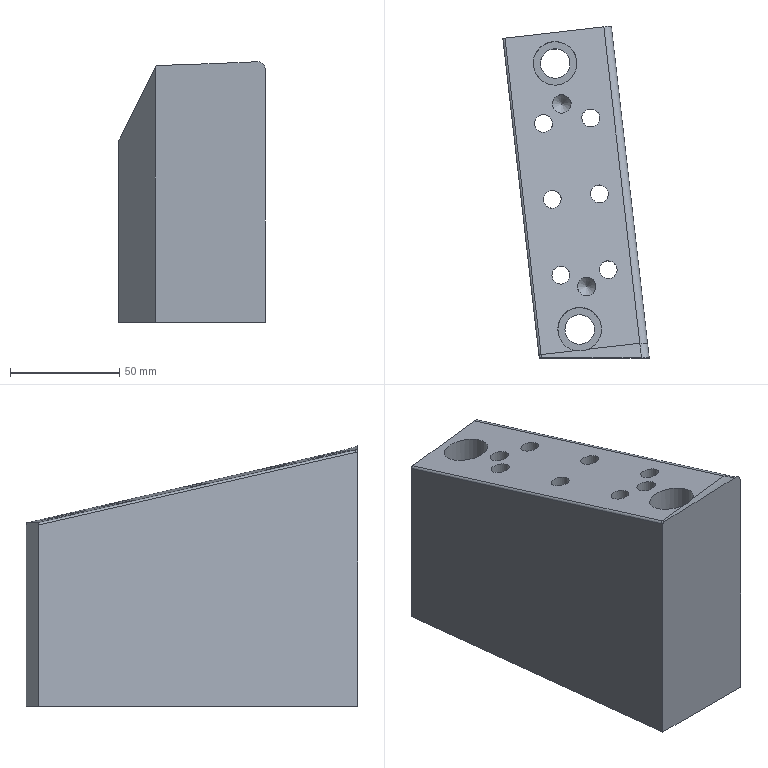Part | NX | features 23 2 | 1 solid | 39 faces | box 66.997 x 151.872 x 119.306 mm | volume 656221 mm3 | cylinder 21 | plane 14 | torus 2 | cone 2 | commonest cylinder face diameters 8.2 x6 10.31 x6 8.5 x2 13.5 x2 20 x2 2 x1
STEP:
#1=CARTESIAN_POINT('',(2421.16,352.401,-62.464));
#2=VERTEX_POINT('',#1);
#3=CARTESIAN_POINT('',(2421.641,348.178,-61.495));
#4=DIRECTION('',(0.02515,-0.2207,-0.975));
#5=DIRECTION('',(-0.1104,0.9687,-0.2221));
#6=AXIS2_PLACEMENT_3D('',#3,#4,#5);
#7=ELLIPSE('',#6,4.359,4.25);
#8=EDGE_CURVE('',#2,#2,#7,.T.);
#9=ORIENTED_EDGE('',*,*,#8,.T.);
#10=EDGE_LOOP('',(#9));
#11=FACE_BOUND('',#10,.T.);
#12=CARTESIAN_POINT('',(2432.577,268.755,-43.235));
#13=VERTEX_POINT('',#12);
#14=CARTESIAN_POINT('',(2433.058,264.532,-42.267));
#15=DIRECTION('',(0.02515,-0.2207,-0.975));
#16=DIRECTION('',(-0.1104,0.9687,-0.2221));
#17=AXIS2_PLACEMENT_3D('',#14,#15,#16);
#18=ELLIPSE('',#17,4.359,4.25);
#19=EDGE_CURVE('',#13,#13,#18,.T.);
#20=ORIENTED_EDGE('',*,*,#19,.T.);
#21=EDGE_LOOP('',(#20));
#22=FACE_BOUND('',#21,.T.);
#23=CARTESIAN_POINT('',(2435.399,337.674,-58.763));
#24=VERTEX_POINT('',#23);
#25=CARTESIAN_POINT('',(2434.935,341.748,-59.697));
#26=DIRECTION('',(-0.02515,0.2207,0.975));
#27=DIRECTION('',(0.1104,-0.9687,0.2221));
#28=AXIS2_PLACEMENT_3D('',#25,#26,#27);
#29=ELLIPSE('',#28,4.205,4.1);
#30=EDGE_CURVE('',#24,#24,#29,.T.);
#31=ORIENTED_EDGE('',*,*,#30,.F.);
#32=EDGE_LOOP('',(#31));
#33=FACE_BOUND('',#32,.T.);
#34=CARTESIAN_POINT('',(2413.764,335.21,-58.763));
#35=VERTEX_POINT('',#34);
#36=CARTESIAN_POINT('',(2413.3,339.283,-59.697));
#37=DIRECTION('',(-0.02515,0.2207,0.975));
#38=DIRECTION('',(0.1104,-0.9687,0.2221));
#39=AXIS2_PLACEMENT_3D('',#36,#37,#38);
#40=ELLIPSE('',#39,4.205,4.1);
#41=EDGE_CURVE('',#35,#35,#40,.T.);
#42=ORIENTED_EDGE('',*,*,#41,.F.);
#43=EDGE_LOOP('',(#42));
#44=FACE_BOUND('',#43,.T.);
#45=CARTESIAN_POINT('',(2439.361,302.899,-50.789));
#46=VERTEX_POINT('',#45);
#47=CARTESIAN_POINT('',(2438.897,306.973,-51.723));
#48=DIRECTION('',(-0.02515,0.2207,0.975));
#49=DIRECTION('',(0.1104,-0.9687,0.2221));
#50=AXIS2_PLACEMENT_3D('',#47,#48,#49);
#51=ELLIPSE('',#50,4.205,4.1);
#52=EDGE_CURVE('',#46,#46,#51,.T.);
#53=ORIENTED_EDGE('',*,*,#52,.F.);
#54=EDGE_LOOP('',(#53));
#55=FACE_BOUND('',#54,.T.);
#56=CARTESIAN_POINT('',(2417.727,300.435,-50.789));
#57=VERTEX_POINT('',#56);
#58=CARTESIAN_POINT('',(2417.262,304.508,-51.723));
#59=DIRECTION('',(-0.02515,0.2207,0.975));
#60=DIRECTION('',(0.1104,-0.9687,0.2221));
#61=AXIS2_PLACEMENT_3D('',#58,#59,#60);
#62=ELLIPSE('',#61,4.205,4.1);
#63=EDGE_CURVE('',#57,#57,#62,.T.);
#64=ORIENTED_EDGE('',*,*,#63,.F.);
#65=EDGE_LOOP('',(#64));
#66=FACE_BOUND('',#65,.T.);
#67=CARTESIAN_POINT('',(2443.323,268.124,-42.815));
#68=VERTEX_POINT('',#67);
#69=CARTESIAN_POINT('',(2442.859,272.198,-43.749));
#70=DIRECTION('',(-0.02515,0.2207,0.975));
#71=DIRECTION('',(0.1104,-0.9687,0.2221));
#72=AXIS2_PLACEMENT_3D('',#69,#70,#71);
#73=ELLIPSE('',#72,4.205,4.1);
#74=EDGE_CURVE('',#68,#68,#73,.T.);
#75=ORIENTED_EDGE('',*,*,#74,.F.);
#76=EDGE_LOOP('',(#75));
#77=FACE_BOUND('',#76,.T.);
#78=CARTESIAN_POINT('',(2421.689,265.66,-42.815));
#79=VERTEX_POINT('',#78);
#80=CARTESIAN_POINT('',(2421.225,269.733,-43.749));
#81=DIRECTION('',(-0.02515,0.2207,0.975));
#82=DIRECTION('',(0.1104,-0.9687,0.2221));
#83=AXIS2_PLACEMENT_3D('',#80,#81,#82);
#84=ELLIPSE('',#83,4.205,4.1);
#85=EDGE_CURVE('',#79,#79,#84,.T.);
#86=ORIENTED_EDGE('',*,*,#85,.F.);
#87=EDGE_LOOP('',(#86));
#88=FACE_BOUND('',#87,.T.);
#89=CARTESIAN_POINT('',(2417.47,376.713,-68.062));
#90=VERTEX_POINT('',#89);
#91=CARTESIAN_POINT('',(2418.602,366.777,-65.784));
#92=DIRECTION('',(-0.02515,0.2207,0.975));
#93=DIRECTION('',(-0.1104,0.9687,-0.2221));
#94=AXIS2_PLACEMENT_3D('',#91,#92,#93);
#95=ELLIPSE('',#94,10.256,10.);
#96=EDGE_CURVE('',#90,#90,#95,.T.);
#97=ORIENTED_EDGE('',*,*,#96,.F.);
#98=EDGE_LOOP('',(#97));
#99=FACE_BOUND('',#98,.T.);
#100=CARTESIAN_POINT('',(2433.88,235.852,-35.754));
#101=VERTEX_POINT('',#100);
#102=CARTESIAN_POINT('',(2457.384,238.53,-35.754));
#103=VERTEX_POINT('',#102);
#104=CARTESIAN_POINT('',(2451.423,237.851,-35.754));
#105=DIRECTION('',(0.9936,0.1132,0.000000001));
#106=VECTOR('',#105,1000.);
#107=LINE('',#104,#106);
#108=EDGE_CURVE('',#101,#103,#107,.T.);
#109=ORIENTED_EDGE('',*,*,#108,.T.);
#110=CARTESIAN_POINT('',(2440.87,383.475,-68.989));
#111=VERTEX_POINT('',#110);
#112=CARTESIAN_POINT('',(2449.818,304.94,-50.981));
#113=DIRECTION('',(-0.1104,0.9687,-0.2221));
#114=VECTOR('',#113,1000.);
#115=LINE('',#112,#114);
#116=EDGE_CURVE('',#103,#111,#115,.T.);
#117=ORIENTED_EDGE('',*,*,#116,.T.);
#118=CARTESIAN_POINT('',(2395.647,378.323,-68.989));
#119=VERTEX_POINT('',#118);
#120=CARTESIAN_POINT('',(2395.583,378.316,-68.989));
#121=DIRECTION('',(0.9936,0.1132,-0.000000001));
#122=VECTOR('',#121,1000.);
#123=LINE('',#120,#122);
#124=EDGE_CURVE('',#119,#111,#123,.T.);
#125=ORIENTED_EDGE('',*,*,#124,.F.);
#126=CARTESIAN_POINT('',(2412.161,233.378,-35.754));
#127=VERTEX_POINT('',#126);
#128=CARTESIAN_POINT('',(2397.033,366.153,-66.199));
#129=DIRECTION('',(-0.1104,0.9687,-0.2221));
#130=VECTOR('',#129,1000.);
#131=LINE('',#128,#130);
#132=EDGE_CURVE('',#127,#119,#131,.T.);
#133=ORIENTED_EDGE('',*,*,#132,.F.);
#134=CARTESIAN_POINT('',(2427.963,235.178,-35.754));
#135=VERTEX_POINT('',#134);
#136=CARTESIAN_POINT('',(2451.423,237.851,-35.754));
#137=DIRECTION('',(0.9936,0.1132,0.000000001));
#138=VECTOR('',#137,1000.);
#139=LINE('',#136,#138);
#140=EDGE_CURVE('',#127,#135,#139,.T.);
#141=ORIENTED_EDGE('',*,*,#140,.T.);
#142=CARTESIAN_POINT('',(2429.841,245.,-37.929));
#143=DIRECTION('',(-0.02515,0.2207,0.975));
#144=DIRECTION('',(-0.1104,0.9687,-0.2221));
#145=AXIS2_PLACEMENT_3D('',#142,#143,#144);
#146=ELLIPSE('',#145,10.256,10.);
#147=EDGE_CURVE('',#101,#135,#146,.T.);
#148=ORIENTED_EDGE('',*,*,#147,.F.);
#149=EDGE_LOOP('',(#109,#117,#125,#133,#141,#148));
#150=FACE_BOUND('',#149,.T.);
#151=CARTESIAN_POINT('',(2449.211,372.098,-66.199));
#152=DIRECTION('',(0.02515,-0.2207,-0.975));
#153=DIRECTION('',(-0.1104,0.9687,-0.2221));
#154=AXIS2_PLACEMENT_3D('',#151,#152,#153);
#155=PLANE('',#154);
#156=ADVANCED_FACE('',(#11,#22,#33,#44,#55,#66,#77,#88,#99,#150),#155,.F.);
#157=CARTESIAN_POINT('',(2394.653,378.21,-70.015));
#158=VERTEX_POINT('',#157);
#159=CARTESIAN_POINT('',(2395.647,378.323,-70.015));
#160=DIRECTION('',(0.1132,-0.9936,0.));
#161=DIRECTION('',(0.,0.,1.));
#162=AXIS2_PLACEMENT_3D('',#159,#160,#161);
#163=ELLIPSE('',#162,1.026,1.);
#164=EDGE_CURVE('',#119,#158,#163,.T.);
#165=ORIENTED_EDGE('',*,*,#164,.F.);
#166=ORIENTED_EDGE('',*,*,#124,.T.);
#167=CARTESIAN_POINT('',(2444.347,383.872,-72.579));
#168=VERTEX_POINT('',#167);
#169=CARTESIAN_POINT('',(2440.87,383.475,-72.579));
#170=DIRECTION('',(0.1132,-0.9936,0.));
#171=DIRECTION('',(0.,0.,1.));
#172=AXIS2_PLACEMENT_3D('',#169,#170,#171);
#173=ELLIPSE('',#172,3.59,3.5);
#174=EDGE_CURVE('',#168,#111,#173,.T.);
#175=ORIENTED_EDGE('',*,*,#174,.F.);
#176=CARTESIAN_POINT('',(2444.347,383.872,-153.));
#177=VERTEX_POINT('',#176);
#178=CARTESIAN_POINT('',(2444.347,383.872,-57.626));
#179=DIRECTION('',(-0.000000001,0.,1.));
#180=VECTOR('',#179,1000.);
#181=LINE('',#178,#180);
#182=EDGE_CURVE('',#177,#168,#181,.T.);
#183=ORIENTED_EDGE('',*,*,#182,.F.);
#184=CARTESIAN_POINT('',(2394.653,378.21,-153.));
#185=VERTEX_POINT('',#184);
#186=CARTESIAN_POINT('',(2395.583,378.316,-153.));
#187=DIRECTION('',(0.9936,0.1132,0.));
#188=VECTOR('',#187,1000.);
#189=LINE('',#186,#188);
#190=EDGE_CURVE('',#185,#177,#189,.T.);
#191=ORIENTED_EDGE('',*,*,#190,.F.);
#192=CARTESIAN_POINT('',(2394.653,378.21,-57.626));
#193=DIRECTION('',(-0.000000002,0.,-1.));
#194=VECTOR('',#193,1000.);
#195=LINE('',#192,#194);
#196=EDGE_CURVE('',#158,#185,#195,.T.);
#197=ORIENTED_EDGE('',*,*,#196,.F.);
#198=EDGE_LOOP('',(#165,#166,#175,#183,#191,#197));
#199=FACE_BOUND('',#198,.T.);
#200=CARTESIAN_POINT('',(2395.583,378.316,-57.626));
#201=DIRECTION('',(-0.1132,0.9936,0.));
#202=DIRECTION('',(0.02514,0.002864,0.9997));
#203=AXIS2_PLACEMENT_3D('',#200,#201,#202);
#204=PLANE('',#203);
#205=ADVANCED_FACE('',(#199),#204,.T.);
#206=CARTESIAN_POINT('',(2411.312,232.,-153.));
#207=VERTEX_POINT('',#206);
#208=CARTESIAN_POINT('',(2411.312,232.,-36.476));
#209=VERTEX_POINT('',#208);
#210=CARTESIAN_POINT('',(2411.312,232.,0.000000275));
#211=DIRECTION('',(0.000000002,0.,1.));
#212=VECTOR('',#211,1000.);
#213=LINE('',#210,#212);
#214=EDGE_CURVE('',#207,#209,#213,.T.);
#215=ORIENTED_EDGE('',*,*,#214,.F.);
#216=CARTESIAN_POINT('',(2461.651,232.,-153.));
#217=VERTEX_POINT('',#216);
#218=CARTESIAN_POINT('',(2566.,232.,-153.));
#219=DIRECTION('',(-1.,0.,0.));
#220=VECTOR('',#219,1000.);
#221=LINE('',#218,#220);
#222=EDGE_CURVE('',#217,#207,#221,.T.);
#223=ORIENTED_EDGE('',*,*,#222,.F.);
#224=CARTESIAN_POINT('',(2461.651,232.,-37.299));
#225=VERTEX_POINT('',#224);
#226=CARTESIAN_POINT('',(2461.651,232.,-0.000000076));
#227=DIRECTION('',(0.000000001,0.,-1.));
#228=VECTOR('',#227,1000.);
#229=LINE('',#226,#228);
#230=EDGE_CURVE('',#225,#217,#229,.T.);
#231=ORIENTED_EDGE('',*,*,#230,.F.);
#232=CARTESIAN_POINT('',(2458.128,232.,-33.697));
#233=VERTEX_POINT('',#232);
#234=CARTESIAN_POINT('',(2458.128,232.,-33.697));
#235=CARTESIAN_POINT('',(2459.076,232.,-33.654));
#236=CARTESIAN_POINT('',(2460.953,232.,-34.457));
#237=CARTESIAN_POINT('',(2461.651,232.,-36.351));
#238=CARTESIAN_POINT('',(2461.651,232.,-37.299));
#239=B_SPLINE_CURVE_WITH_KNOTS('',3,(#234,#235,#236,#237,#238),.UNSPECIFIED.,.F.,.F.,(4,1,4),(0.,0.002806,0.005613),.UNSPECIFIED.);
#240=EDGE_CURVE('',#233,#225,#239,.T.);
#241=ORIENTED_EDGE('',*,*,#240,.F.);
#242=CARTESIAN_POINT('',(2412.318,232.,-35.414));
#243=VERTEX_POINT('',#242);
#244=CARTESIAN_POINT('',(2314.714,232.,6.659));
#245=DIRECTION('',(0.,1.,0.));
#246=DIRECTION('',(1.,0.,0.000000001));
#247=AXIS2_PLACEMENT_3D('',#244,#245,#246);
#248=ELLIPSE('',#247,384.265,43.5);
#249=EDGE_CURVE('',#233,#243,#248,.T.);
#250=ORIENTED_EDGE('',*,*,#249,.T.);
#251=CARTESIAN_POINT('',(2411.312,232.,-36.476));
#252=CARTESIAN_POINT('',(2411.312,232.,-35.932));
#253=CARTESIAN_POINT('',(2411.774,232.,-35.43));
#254=CARTESIAN_POINT('',(2412.318,232.,-35.414));
#255=B_SPLINE_CURVE_WITH_KNOTS('',3,(#251,#252,#253,#254),.UNSPECIFIED.,.F.,.F.,(4,4),(0.,0.001608),.UNSPECIFIED.);
#256=EDGE_CURVE('',#209,#243,#255,.T.);
#257=ORIENTED_EDGE('',*,*,#256,.F.);
#258=EDGE_LOOP('',(#215,#223,#231,#241,#250,#257));
#259=FACE_BOUND('',#258,.T.);
#260=CARTESIAN_POINT('',(2566.,232.,0.));
#261=DIRECTION('',(0.,-1.,0.));
#262=DIRECTION('',(0.,0.,-1.));
#263=AXIS2_PLACEMENT_3D('',#260,#261,#262);
#264=PLANE('',#263);
#265=ADVANCED_FACE('',(#259),#264,.T.);
#266=CARTESIAN_POINT('',(2429.78,341.748,-153.));
#267=VERTEX_POINT('',#266);
#268=CARTESIAN_POINT('',(2434.935,341.748,-153.));
#269=DIRECTION('',(0.,0.,1.));
#270=DIRECTION('',(-1.,0.,0.));
#271=AXIS2_PLACEMENT_3D('',#268,#269,#270);
#272=CIRCLE('',#271,5.155);
#273=EDGE_CURVE('',#267,#267,#272,.T.);
#274=ORIENTED_EDGE('',*,*,#273,.T.);
#275=EDGE_LOOP('',(#274));
#276=FACE_BOUND('',#275,.T.);
#277=CARTESIAN_POINT('',(2408.145,339.283,-153.));
#278=VERTEX_POINT('',#277);
#279=CARTESIAN_POINT('',(2413.3,339.283,-153.));
#280=DIRECTION('',(0.,0.,1.));
#281=DIRECTION('',(-1.,0.,0.));
#282=AXIS2_PLACEMENT_3D('',#279,#280,#281);
#283=CIRCLE('',#282,5.155);
#284=EDGE_CURVE('',#278,#278,#283,.T.);
#285=ORIENTED_EDGE('',*,*,#284,.T.);
#286=EDGE_LOOP('',(#285));
#287=FACE_BOUND('',#286,.T.);
#288=CARTESIAN_POINT('',(2433.742,306.973,-153.));
#289=VERTEX_POINT('',#288);
#290=CARTESIAN_POINT('',(2438.897,306.973,-153.));
#291=DIRECTION('',(0.,0.,1.));
#292=DIRECTION('',(-1.,0.,0.));
#293=AXIS2_PLACEMENT_3D('',#290,#291,#292);
#294=CIRCLE('',#293,5.155);
#295=EDGE_CURVE('',#289,#289,#294,.T.);
#296=ORIENTED_EDGE('',*,*,#295,.T.);
#297=EDGE_LOOP('',(#296));
#298=FACE_BOUND('',#297,.T.);
#299=CARTESIAN_POINT('',(2412.107,304.508,-153.));
#300=VERTEX_POINT('',#299);
#301=CARTESIAN_POINT('',(2417.262,304.508,-153.));
#302=DIRECTION('',(0.,0.,1.));
#303=DIRECTION('',(-1.,0.,0.));
#304=AXIS2_PLACEMENT_3D('',#301,#302,#303);
#305=CIRCLE('',#304,5.155);
#306=EDGE_CURVE('',#300,#300,#305,.T.);
#307=ORIENTED_EDGE('',*,*,#306,.T.);
#308=EDGE_LOOP('',(#307));
#309=FACE_BOUND('',#308,.T.);
#310=CARTESIAN_POINT('',(2437.704,272.198,-153.));
#311=VERTEX_POINT('',#310);
#312=CARTESIAN_POINT('',(2442.859,272.198,-153.));
#313=DIRECTION('',(0.,0.,1.));
#314=DIRECTION('',(-1.,0.,0.));
#315=AXIS2_PLACEMENT_3D('',#312,#313,#314);
#316=CIRCLE('',#315,5.155);
#317=EDGE_CURVE('',#311,#311,#316,.T.);
#318=ORIENTED_EDGE('',*,*,#317,.T.);
#319=EDGE_LOOP('',(#318));
#320=FACE_BOUND('',#319,.T.);
#321=CARTESIAN_POINT('',(2416.07,269.733,-153.));
#322=VERTEX_POINT('',#321);
#323=CARTESIAN_POINT('',(2421.225,269.733,-153.));
#324=DIRECTION('',(0.,0.,1.));
#325=DIRECTION('',(-1.,0.,0.));
#326=AXIS2_PLACEMENT_3D('',#323,#324,#325);
#327=CIRCLE('',#326,5.155);
#328=EDGE_CURVE('',#322,#322,#327,.T.);
#329=ORIENTED_EDGE('',*,*,#328,.T.);
#330=EDGE_LOOP('',(#329));
#331=FACE_BOUND('',#330,.T.);
#332=CARTESIAN_POINT('',(2411.852,366.777,-153.));
#333=VERTEX_POINT('',#332);
#334=CARTESIAN_POINT('',(2418.602,366.777,-153.));
#335=DIRECTION('',(0.,0.,1.));
#336=DIRECTION('',(-1.,0.,0.));
#337=AXIS2_PLACEMENT_3D('',#334,#335,#336);
#338=CIRCLE('',#337,6.75);
#339=EDGE_CURVE('',#333,#333,#338,.T.);
#340=ORIENTED_EDGE('',*,*,#339,.T.);
#341=EDGE_LOOP('',(#340));
#342=FACE_BOUND('',#341,.T.);
#343=CARTESIAN_POINT('',(2423.091,245.,-153.));
#344=VERTEX_POINT('',#343);
#345=CARTESIAN_POINT('',(2429.841,245.,-153.));
#346=DIRECTION('',(0.,0.,1.));
#347=DIRECTION('',(-1.,0.,0.));
#348=AXIS2_PLACEMENT_3D('',#345,#346,#347);
#349=CIRCLE('',#348,6.75);
#350=EDGE_CURVE('',#344,#344,#349,.T.);
#351=ORIENTED_EDGE('',*,*,#350,.T.);
#352=EDGE_LOOP('',(#351));
#353=FACE_BOUND('',#352,.T.);
#354=ORIENTED_EDGE('',*,*,#190,.T.);
#355=CARTESIAN_POINT('',(2481.527,57.547,-153.));
#356=DIRECTION('',(-0.1132,0.9936,0.));
#357=VECTOR('',#356,1000.);
#358=LINE('',#355,#357);
#359=EDGE_CURVE('',#217,#177,#358,.T.);
#360=ORIENTED_EDGE('',*,*,#359,.F.);
#361=ORIENTED_EDGE('',*,*,#222,.T.);
#362=CARTESIAN_POINT('',(2431.833,51.886,-153.));
#363=DIRECTION('',(0.1132,-0.9936,0.));
#364=VECTOR('',#363,1000.);
#365=LINE('',#362,#364);
#366=EDGE_CURVE('',#185,#207,#365,.T.);
#367=ORIENTED_EDGE('',*,*,#366,.F.);
#368=EDGE_LOOP('',(#354,#360,#361,#367));
#369=FACE_BOUND('',#368,.T.);
#370=CARTESIAN_POINT('',(282.5,-193.,-153.));
#371=DIRECTION('',(0.,0.,-1.));
#372=DIRECTION('',(-1.,0.,0.));
#373=AXIS2_PLACEMENT_3D('',#370,#371,#372);
#374=PLANE('',#373);
#375=ADVANCED_FACE('',(#276,#287,#298,#309,#320,#331,#342,#353,#369),#374,.T.);
#376=ORIENTED_EDGE('',*,*,#132,.T.);
#377=ORIENTED_EDGE('',*,*,#164,.T.);
#378=CARTESIAN_POINT('',(2411.193,233.044,-36.729));
#379=VERTEX_POINT('',#378);
#380=CARTESIAN_POINT('',(2396.065,365.819,-67.174));
#381=DIRECTION('',(0.1104,-0.9687,0.2221));
#382=VECTOR('',#381,1000.);
#383=LINE('',#380,#382);
#384=EDGE_CURVE('',#158,#379,#383,.T.);
#385=ORIENTED_EDGE('',*,*,#384,.T.);
#386=CARTESIAN_POINT('',(2412.186,233.157,-36.729));
#387=DIRECTION('',(0.1104,-0.9687,0.2221));
#388=DIRECTION('',(0.,-0.2235,-0.9747));
#389=AXIS2_PLACEMENT_3D('',#386,#387,#388);
#390=CIRCLE('',#389,1.);
#391=EDGE_CURVE('',#127,#379,#390,.T.);
#392=ORIENTED_EDGE('',*,*,#391,.F.);
#393=EDGE_LOOP('',(#376,#377,#385,#392));
#394=FACE_BOUND('',#393,.T.);
#395=CARTESIAN_POINT('',(2397.059,365.932,-67.174));
#396=DIRECTION('',(0.1104,-0.9687,0.2221));
#397=DIRECTION('',(0.,0.2235,0.9747));
#398=AXIS2_PLACEMENT_3D('',#395,#396,#397);
#399=CYLINDRICAL_SURFACE('',#398,1.);
#400=ADVANCED_FACE('',(#394),#399,.T.);
#401=CARTESIAN_POINT('',(2410.074,242.865,6.659));
#402=DIRECTION('',(-0.9936,-0.1132,0.000000002));
#403=DIRECTION('',(-0.1132,0.9936,0.));
#404=AXIS2_PLACEMENT_3D('',#401,#402,#403);
#405=CIRCLE('',#404,44.5);
#406=EDGE_CURVE('',#379,#209,#405,.T.);
#407=ORIENTED_EDGE('',*,*,#406,.F.);
#408=ORIENTED_EDGE('',*,*,#384,.F.);
#409=ORIENTED_EDGE('',*,*,#196,.T.);
#410=ORIENTED_EDGE('',*,*,#366,.T.);
#411=ORIENTED_EDGE('',*,*,#214,.T.);
#412=EDGE_LOOP('',(#407,#408,#409,#410,#411));
#413=FACE_BOUND('',#412,.T.);
#414=CARTESIAN_POINT('',(2411.08,234.037,-32.341));
#415=DIRECTION('',(-0.9936,-0.1132,0.000000002));
#416=DIRECTION('',(0.1132,-0.9936,0.000000002));
#417=AXIS2_PLACEMENT_3D('',#414,#415,#416);
#418=PLANE('',#417);
#419=ADVANCED_FACE('',(#413),#418,.T.);
#420=ORIENTED_EDGE('',*,*,#174,.T.);
#421=ORIENTED_EDGE('',*,*,#116,.F.);
#422=CARTESIAN_POINT('',(2460.95,238.154,-39.166));
#423=VERTEX_POINT('',#422);
#424=CARTESIAN_POINT('',(2457.472,237.758,-39.166));
#425=DIRECTION('',(-0.1104,0.9687,-0.2221));
#426=DIRECTION('',(-0.6687,-0.2377,-0.7045));
#427=AXIS2_PLACEMENT_3D('',#424,#425,#426);
#428=CIRCLE('',#427,3.5);
#429=EDGE_CURVE('',#103,#423,#428,.T.);
#430=ORIENTED_EDGE('',*,*,#429,.T.);
#431=CARTESIAN_POINT('',(2453.383,304.563,-54.394));
#432=DIRECTION('',(0.1104,-0.9687,0.2221));
#433=VECTOR('',#432,1000.);
#434=LINE('',#431,#433);
#435=EDGE_CURVE('',#168,#423,#434,.T.);
#436=ORIENTED_EDGE('',*,*,#435,.F.);
#437=EDGE_LOOP('',(#420,#421,#430,#436));
#438=FACE_BOUND('',#437,.T.);
#439=CARTESIAN_POINT('',(2452.744,279.254,-48.681));
#440=DIRECTION('',(0.1104,-0.9687,0.2221));
#441=DIRECTION('',(0.6848,0.2361,0.6894));
#442=AXIS2_PLACEMENT_3D('',#439,#440,#441);
#443=CYLINDRICAL_SURFACE('',#442,3.5);
#444=ADVANCED_FACE('',(#438),#443,.T.);
#445=ORIENTED_EDGE('',*,*,#435,.T.);
#446=CARTESIAN_POINT('',(2463.469,216.037,-27.1));
#447=CARTESIAN_POINT('',(2462.948,220.611,-31.559));
#448=CARTESIAN_POINT('',(2462.335,225.992,-35.182));
#449=CARTESIAN_POINT('',(2461.657,231.945,-37.743));
#450=CARTESIAN_POINT('',(2460.95,238.154,-39.166));
#451=B_SPLINE_CURVE_WITH_KNOTS('',4,(#446,#447,#448,#449,#450),.UNSPECIFIED.,.F.,.F.,(5,5),(0.,1.),.PIECEWISE_BEZIER_KNOTS.);
#452=EDGE_CURVE('',#225,#423,#451,.T.);
#453=ORIENTED_EDGE('',*,*,#452,.F.);
#454=ORIENTED_EDGE('',*,*,#230,.T.);
#455=ORIENTED_EDGE('',*,*,#359,.T.);
#456=ORIENTED_EDGE('',*,*,#182,.T.);
#457=EDGE_LOOP('',(#445,#453,#454,#455,#456));
#458=FACE_BOUND('',#457,.T.);
#459=CARTESIAN_POINT('',(2310.296,1560.421,-706.6));
#460=DIRECTION('',(0.9936,0.1132,0.000000001));
#461=DIRECTION('',(0.000000001,-0.000000001,-1.));
#462=AXIS2_PLACEMENT_3D('',#459,#460,#461);
#463=PLANE('',#462);
#464=ADVANCED_FACE('',(#458),#463,.T.);
#465=ORIENTED_EDGE('',*,*,#256,.T.);
#466=CARTESIAN_POINT('',(2412.318,232.,-35.414));
#467=CARTESIAN_POINT('',(2412.266,232.457,-35.535));
#468=CARTESIAN_POINT('',(2412.214,232.916,-35.648));
#469=CARTESIAN_POINT('',(2412.161,233.378,-35.754));
#470=B_SPLINE_CURVE_WITH_KNOTS('',3,(#466,#467,#468,#469),.UNSPECIFIED.,.F.,.F.,(4,4),(0.,1.),.PIECEWISE_BEZIER_KNOTS.);
#471=EDGE_CURVE('',#243,#127,#470,.T.);
#472=ORIENTED_EDGE('',*,*,#471,.T.);
#473=ORIENTED_EDGE('',*,*,#391,.T.);
#474=ORIENTED_EDGE('',*,*,#406,.T.);
#475=EDGE_LOOP('',(#465,#472,#473,#474));
#476=FACE_BOUND('',#475,.T.);
#477=CARTESIAN_POINT('',(2411.067,242.978,6.659));
#478=DIRECTION('',(-0.9936,-0.1132,0.000000002));
#479=DIRECTION('',(0.1132,-0.9936,0.));
#480=AXIS2_PLACEMENT_3D('',#477,#478,#479);
#481=TOROIDAL_SURFACE('',#480,44.5,1.);
#482=ADVANCED_FACE('',(#476),#481,.T.);
#483=ORIENTED_EDGE('',*,*,#240,.T.);
#484=ORIENTED_EDGE('',*,*,#452,.T.);
#485=ORIENTED_EDGE('',*,*,#429,.F.);
#486=CARTESIAN_POINT('',(2456.29,248.131,6.659));
#487=DIRECTION('',(-0.9936,-0.1132,-0.000000001));
#488=DIRECTION('',(0.1132,-0.9936,0.000000001));
#489=AXIS2_PLACEMENT_3D('',#486,#487,#488);
#490=CIRCLE('',#489,43.5);
#491=EDGE_CURVE('',#103,#233,#490,.T.);
#492=ORIENTED_EDGE('',*,*,#491,.T.);
#493=EDGE_LOOP('',(#483,#484,#485,#492));
#494=FACE_BOUND('',#493,.T.);
#495=CARTESIAN_POINT('',(2456.29,248.131,6.659));
#496=DIRECTION('',(0.9936,0.1132,0.000000001));
#497=DIRECTION('',(0.05395,-0.4735,-0.8791));
#498=AXIS2_PLACEMENT_3D('',#495,#496,#497);
#499=TOROIDAL_SURFACE('',#498,47.,3.5);
#500=ADVANCED_FACE('',(#494),#499,.T.);
#501=ORIENTED_EDGE('',*,*,#140,.F.);
#502=ORIENTED_EDGE('',*,*,#471,.F.);
#503=ORIENTED_EDGE('',*,*,#249,.F.);
#504=ORIENTED_EDGE('',*,*,#491,.F.);
#505=ORIENTED_EDGE('',*,*,#108,.F.);
#506=CARTESIAN_POINT('',(2427.963,235.178,-35.754));
#507=CARTESIAN_POINT('',(2429.956,234.797,-35.616));
#508=CARTESIAN_POINT('',(2432.024,235.032,-35.616));
#509=CARTESIAN_POINT('',(2433.88,235.852,-35.754));
#510=B_SPLINE_CURVE_WITH_KNOTS('',3,(#506,#507,#508,#509),.UNSPECIFIED.,.F.,.F.,(4,4),(0.,0.006016),.UNSPECIFIED.);
#511=EDGE_CURVE('',#135,#101,#510,.T.);
#512=ORIENTED_EDGE('',*,*,#511,.F.);
#513=EDGE_LOOP('',(#501,#502,#503,#504,#505,#512));
#514=FACE_BOUND('',#513,.T.);
#515=CARTESIAN_POINT('',(2445.361,246.885,6.659));
#516=DIRECTION('',(0.9936,0.1132,0.000000001));
#517=DIRECTION('',(0.08782,-0.7708,-0.631));
#518=AXIS2_PLACEMENT_3D('',#515,#516,#517);
#519=CYLINDRICAL_SURFACE('',#518,43.5);
#520=ADVANCED_FACE('',(#514),#519,.F.);
#521=CARTESIAN_POINT('',(2439.841,245.,-123.));
#522=VERTEX_POINT('',#521);
#523=CARTESIAN_POINT('',(2429.841,245.,-123.));
#524=DIRECTION('',(0.,0.,1.));
#525=DIRECTION('',(1.,0.,0.));
#526=AXIS2_PLACEMENT_3D('',#523,#524,#525);
#527=CIRCLE('',#526,10.);
#528=EDGE_CURVE('',#522,#522,#527,.T.);
#529=ORIENTED_EDGE('',*,*,#528,.F.);
#530=EDGE_LOOP('',(#529));
#531=FACE_BOUND('',#530,.T.);
#532=ORIENTED_EDGE('',*,*,#511,.T.);
#533=ORIENTED_EDGE('',*,*,#147,.T.);
#534=EDGE_LOOP('',(#532,#533));
#535=FACE_BOUND('',#534,.T.);
#536=CARTESIAN_POINT('',(2429.841,245.,-33.507));
#537=DIRECTION('',(0.,0.,-1.));
#538=DIRECTION('',(-1.,0.,0.));
#539=AXIS2_PLACEMENT_3D('',#536,#537,#538);
#540=CYLINDRICAL_SURFACE('',#539,10.);
#541=ADVANCED_FACE('',(#531,#535),#540,.F.);
#542=ORIENTED_EDGE('',*,*,#350,.F.);
#543=EDGE_LOOP('',(#542));
#544=FACE_BOUND('',#543,.T.);
#545=CARTESIAN_POINT('',(2436.591,245.,-123.));
#546=VERTEX_POINT('',#545);
#547=CARTESIAN_POINT('',(2429.841,245.,-123.));
#548=DIRECTION('',(0.,0.,1.));
#549=DIRECTION('',(1.,0.,0.));
#550=AXIS2_PLACEMENT_3D('',#547,#548,#549);
#551=CIRCLE('',#550,6.75);
#552=EDGE_CURVE('',#546,#546,#551,.T.);
#553=ORIENTED_EDGE('',*,*,#552,.T.);
#554=EDGE_LOOP('',(#553));
#555=FACE_BOUND('',#554,.T.);
#556=CARTESIAN_POINT('',(2429.841,245.,-28.507));
#557=DIRECTION('',(0.,0.,-1.));
#558=DIRECTION('',(-1.,0.,0.));
#559=AXIS2_PLACEMENT_3D('',#556,#557,#558);
#560=CYLINDRICAL_SURFACE('',#559,6.75);
#561=ADVANCED_FACE('',(#544,#555),#560,.F.);
#562=ORIENTED_EDGE('',*,*,#552,.F.);
#563=EDGE_LOOP('',(#562));
#564=FACE_BOUND('',#563,.T.);
#565=ORIENTED_EDGE('',*,*,#528,.T.);
#566=EDGE_LOOP('',(#565));
#567=FACE_BOUND('',#566,.T.);
#568=CARTESIAN_POINT('',(2429.841,245.,-123.));
#569=DIRECTION('',(0.,0.,-1.));
#570=DIRECTION('',(-1.,0.,0.));
#571=AXIS2_PLACEMENT_3D('',#568,#569,#570);
#572=PLANE('',#571);
#573=ADVANCED_FACE('',(#564,#567),#572,.F.);
#574=CARTESIAN_POINT('',(2428.602,366.777,-123.));
#575=VERTEX_POINT('',#574);
#576=CARTESIAN_POINT('',(2418.602,366.777,-123.));
#577=DIRECTION('',(0.,0.,1.));
#578=DIRECTION('',(1.,0.,0.));
#579=AXIS2_PLACEMENT_3D('',#576,#577,#578);
#580=CIRCLE('',#579,10.);
#581=EDGE_CURVE('',#575,#575,#580,.T.);
#582=ORIENTED_EDGE('',*,*,#581,.F.);
#583=EDGE_LOOP('',(#582));
#584=FACE_BOUND('',#583,.T.);
#585=ORIENTED_EDGE('',*,*,#96,.T.);
#586=EDGE_LOOP('',(#585));
#587=FACE_BOUND('',#586,.T.);
#588=CARTESIAN_POINT('',(2418.602,366.777,-33.507));
#589=DIRECTION('',(0.,0.,-1.));
#590=DIRECTION('',(-1.,0.,0.));
#591=AXIS2_PLACEMENT_3D('',#588,#589,#590);
#592=CYLINDRICAL_SURFACE('',#591,10.);
#593=ADVANCED_FACE('',(#584,#587),#592,.F.);
#594=ORIENTED_EDGE('',*,*,#339,.F.);
#595=EDGE_LOOP('',(#594));
#596=FACE_BOUND('',#595,.T.);
#597=CARTESIAN_POINT('',(2425.352,366.777,-123.));
#598=VERTEX_POINT('',#597);
#599=CARTESIAN_POINT('',(2418.602,366.777,-123.));
#600=DIRECTION('',(0.,0.,1.));
#601=DIRECTION('',(1.,0.,0.));
#602=AXIS2_PLACEMENT_3D('',#599,#600,#601);
#603=CIRCLE('',#602,6.75);
#604=EDGE_CURVE('',#598,#598,#603,.T.);
#605=ORIENTED_EDGE('',*,*,#604,.T.);
#606=EDGE_LOOP('',(#605));
#607=FACE_BOUND('',#606,.T.);
#608=CARTESIAN_POINT('',(2418.602,366.777,-28.507));
#609=DIRECTION('',(0.,0.,-1.));
#610=DIRECTION('',(-1.,0.,0.));
#611=AXIS2_PLACEMENT_3D('',#608,#609,#610);
#612=CYLINDRICAL_SURFACE('',#611,6.75);
#613=ADVANCED_FACE('',(#596,#607),#612,.F.);
#614=ORIENTED_EDGE('',*,*,#604,.F.);
#615=EDGE_LOOP('',(#614));
#616=FACE_BOUND('',#615,.T.);
#617=ORIENTED_EDGE('',*,*,#581,.T.);
#618=EDGE_LOOP('',(#617));
#619=FACE_BOUND('',#618,.T.);
#620=CARTESIAN_POINT('',(2418.602,366.777,-123.));
#621=DIRECTION('',(0.,0.,-1.));
#622=DIRECTION('',(-1.,0.,0.));
#623=AXIS2_PLACEMENT_3D('',#620,#621,#622);
#624=PLANE('',#623);
#625=ADVANCED_FACE('',(#616,#619),#624,.F.);
#626=CARTESIAN_POINT('',(2417.125,269.733,-72.8));
#627=VERTEX_POINT('',#626);
#628=CARTESIAN_POINT('',(2421.225,269.733,-72.8));
#629=DIRECTION('',(0.000000001,0.,-1.));
#630=DIRECTION('',(-1.,0.000000001,-0.000000001));
#631=AXIS2_PLACEMENT_3D('',#628,#629,#630);
#632=CIRCLE('',#631,4.1);
#633=EDGE_CURVE('',#627,#627,#632,.T.);
#634=ORIENTED_EDGE('',*,*,#633,.T.);
#635=EDGE_LOOP('',(#634));
#636=FACE_BOUND('',#635,.T.);
#637=ORIENTED_EDGE('',*,*,#85,.T.);
#638=EDGE_LOOP('',(#637));
#639=FACE_BOUND('',#638,.T.);
#640=CARTESIAN_POINT('',(2421.225,269.733,-75.8));
#641=DIRECTION('',(-0.000000001,0.,1.));
#642=DIRECTION('',(1.,-0.000000001,0.000000001));
#643=AXIS2_PLACEMENT_3D('',#640,#641,#642);
#644=CYLINDRICAL_SURFACE('',#643,4.1);
#645=ADVANCED_FACE('',(#636,#639),#644,.F.);
#646=ORIENTED_EDGE('',*,*,#633,.F.);
#647=EDGE_LOOP('',(#646));
#648=FACE_BOUND('',#647,.T.);
#649=CARTESIAN_POINT('',(2426.38,269.733,-72.8));
#650=VERTEX_POINT('',#649);
#651=CARTESIAN_POINT('',(2421.225,269.733,-72.8));
#652=DIRECTION('',(0.000000001,0.,-1.));
#653=DIRECTION('',(1.,0.,0.000000001));
#654=AXIS2_PLACEMENT_3D('',#651,#652,#653);
#655=CIRCLE('',#654,5.155);
#656=EDGE_CURVE('',#650,#650,#655,.T.);
#657=ORIENTED_EDGE('',*,*,#656,.T.);
#658=EDGE_LOOP('',(#657));
#659=FACE_BOUND('',#658,.T.);
#660=CARTESIAN_POINT('',(2421.225,269.733,-72.8));
#661=DIRECTION('',(-0.000000001,0.,1.));
#662=DIRECTION('',(1.,-0.000000001,0.000000001));
#663=AXIS2_PLACEMENT_3D('',#660,#661,#662);
#664=PLANE('',#663);
#665=ADVANCED_FACE('',(#648,#659),#664,.F.);
#666=ORIENTED_EDGE('',*,*,#328,.F.);
#667=EDGE_LOOP('',(#666));
#668=FACE_BOUND('',#667,.T.);
#669=ORIENTED_EDGE('',*,*,#656,.F.);
#670=EDGE_LOOP('',(#669));
#671=FACE_BOUND('',#670,.T.);
#672=CARTESIAN_POINT('',(2421.225,269.733,-72.8));
#673=DIRECTION('',(0.000000001,0.,-1.));
#674=DIRECTION('',(1.,-0.000000001,0.000000001));
#675=AXIS2_PLACEMENT_3D('',#672,#673,#674);
#676=CYLINDRICAL_SURFACE('',#675,5.155);
#677=ADVANCED_FACE('',(#668,#671),#676,.F.);
#678=CARTESIAN_POINT('',(2446.854,273.12,-72.8));
#679=VERTEX_POINT('',#678);
#680=CARTESIAN_POINT('',(2442.859,272.198,-72.8));
#681=DIRECTION('',(0.,0.,1.));
#682=DIRECTION('',(0.9744,0.225,0.));
#683=AXIS2_PLACEMENT_3D('',#680,#681,#682);
#684=CIRCLE('',#683,4.1);
#685=EDGE_CURVE('',#679,#679,#684,.T.);
#686=ORIENTED_EDGE('',*,*,#685,.F.);
#687=EDGE_LOOP('',(#686));
#688=FACE_BOUND('',#687,.T.);
#689=ORIENTED_EDGE('',*,*,#74,.T.);
#690=EDGE_LOOP('',(#689));
#691=FACE_BOUND('',#690,.T.);
#692=CARTESIAN_POINT('',(2442.859,272.198,-75.8));
#693=DIRECTION('',(0.,0.,1.));
#694=DIRECTION('',(-0.9744,-0.225,0.));
#695=AXIS2_PLACEMENT_3D('',#692,#693,#694);
#696=CYLINDRICAL_SURFACE('',#695,4.1);
#697=ADVANCED_FACE('',(#688,#691),#696,.F.);
#698=ORIENTED_EDGE('',*,*,#685,.T.);
#699=EDGE_LOOP('',(#698));
#700=FACE_BOUND('',#699,.T.);
#701=CARTESIAN_POINT('',(2448.014,272.198,-72.8));
#702=VERTEX_POINT('',#701);
#703=CARTESIAN_POINT('',(2442.859,272.198,-72.8));
#704=DIRECTION('',(0.,0.,1.));
#705=DIRECTION('',(1.,0.,0.));
#706=AXIS2_PLACEMENT_3D('',#703,#704,#705);
#707=CIRCLE('',#706,5.155);
#708=EDGE_CURVE('',#702,#702,#707,.T.);
#709=ORIENTED_EDGE('',*,*,#708,.F.);
#710=EDGE_LOOP('',(#709));
#711=FACE_BOUND('',#710,.T.);
#712=CARTESIAN_POINT('',(2442.859,272.198,-72.8));
#713=DIRECTION('',(0.,0.,1.));
#714=DIRECTION('',(-0.9744,-0.225,0.));
#715=AXIS2_PLACEMENT_3D('',#712,#713,#714);
#716=PLANE('',#715);
#717=ADVANCED_FACE('',(#700,#711),#716,.F.);
#718=ORIENTED_EDGE('',*,*,#317,.F.);
#719=EDGE_LOOP('',(#718));
#720=FACE_BOUND('',#719,.T.);
#721=ORIENTED_EDGE('',*,*,#708,.T.);
#722=EDGE_LOOP('',(#721));
#723=FACE_BOUND('',#722,.T.);
#724=CARTESIAN_POINT('',(2442.859,272.198,-72.8));
#725=DIRECTION('',(0.,0.,-1.));
#726=DIRECTION('',(-0.9744,-0.225,0.));
#727=AXIS2_PLACEMENT_3D('',#724,#725,#726);
#728=CYLINDRICAL_SURFACE('',#727,5.155);
#729=ADVANCED_FACE('',(#720,#723),#728,.F.);
#730=CARTESIAN_POINT('',(2413.267,303.586,-80.8));
#731=VERTEX_POINT('',#730);
#732=CARTESIAN_POINT('',(2417.262,304.508,-80.8));
#733=DIRECTION('',(-0.000000001,0.,1.));
#734=DIRECTION('',(-0.9744,-0.225,-0.000000001));
#735=AXIS2_PLACEMENT_3D('',#732,#733,#734);
#736=CIRCLE('',#735,4.1);
#737=EDGE_CURVE('',#731,#731,#736,.T.);
#738=ORIENTED_EDGE('',*,*,#737,.F.);
#739=EDGE_LOOP('',(#738));
#740=FACE_BOUND('',#739,.T.);
#741=ORIENTED_EDGE('',*,*,#63,.T.);
#742=EDGE_LOOP('',(#741));
#743=FACE_BOUND('',#742,.T.);
#744=CARTESIAN_POINT('',(2417.262,304.508,-83.8));
#745=DIRECTION('',(-0.000000001,0.,1.));
#746=DIRECTION('',(0.9744,0.225,0.000000001));
#747=AXIS2_PLACEMENT_3D('',#744,#745,#746);
#748=CYLINDRICAL_SURFACE('',#747,4.1);
#749=ADVANCED_FACE('',(#740,#743),#748,.F.);
#750=ORIENTED_EDGE('',*,*,#737,.T.);
#751=EDGE_LOOP('',(#750));
#752=FACE_BOUND('',#751,.T.);
#753=CARTESIAN_POINT('',(2422.417,304.508,-80.8));
#754=VERTEX_POINT('',#753);
#755=CARTESIAN_POINT('',(2417.262,304.508,-80.8));
#756=DIRECTION('',(-0.000000001,0.,1.));
#757=DIRECTION('',(1.,0.,0.000000001));
#758=AXIS2_PLACEMENT_3D('',#755,#756,#757);
#759=CIRCLE('',#758,5.155);
#760=EDGE_CURVE('',#754,#754,#759,.T.);
#761=ORIENTED_EDGE('',*,*,#760,.F.);
#762=EDGE_LOOP('',(#761));
#763=FACE_BOUND('',#762,.T.);
#764=CARTESIAN_POINT('',(2417.262,304.508,-80.8));
#765=DIRECTION('',(-0.000000001,0.,1.));
#766=DIRECTION('',(0.9744,0.225,0.000000001));
#767=AXIS2_PLACEMENT_3D('',#764,#765,#766);
#768=PLANE('',#767);
#769=ADVANCED_FACE('',(#752,#763),#768,.F.);
#770=ORIENTED_EDGE('',*,*,#306,.F.);
#771=EDGE_LOOP('',(#770));
#772=FACE_BOUND('',#771,.T.);
#773=ORIENTED_EDGE('',*,*,#760,.T.);
#774=EDGE_LOOP('',(#773));
#775=FACE_BOUND('',#774,.T.);
#776=CARTESIAN_POINT('',(2417.262,304.508,-80.8));
#777=DIRECTION('',(0.000000001,0.,-1.));
#778=DIRECTION('',(0.9744,0.225,0.000000001));
#779=AXIS2_PLACEMENT_3D('',#776,#777,#778);
#780=CYLINDRICAL_SURFACE('',#779,5.155);
#781=ADVANCED_FACE('',(#772,#775),#780,.F.);
#782=CARTESIAN_POINT('',(2442.997,306.973,-80.8));
#783=VERTEX_POINT('',#782);
#784=CARTESIAN_POINT('',(2438.897,306.973,-80.8));
#785=DIRECTION('',(0.,0.,-1.));
#786=DIRECTION('',(1.,0.,0.));
#787=AXIS2_PLACEMENT_3D('',#784,#785,#786);
#788=CIRCLE('',#787,4.1);
#789=EDGE_CURVE('',#783,#783,#788,.T.);
#790=ORIENTED_EDGE('',*,*,#789,.T.);
#791=EDGE_LOOP('',(#790));
#792=FACE_BOUND('',#791,.T.);
#793=ORIENTED_EDGE('',*,*,#52,.T.);
#794=EDGE_LOOP('',(#793));
#795=FACE_BOUND('',#794,.T.);
#796=CARTESIAN_POINT('',(2438.897,306.973,-83.8));
#797=DIRECTION('',(0.,0.,1.));
#798=DIRECTION('',(-1.,0.,0.));
#799=AXIS2_PLACEMENT_3D('',#796,#797,#798);
#800=CYLINDRICAL_SURFACE('',#799,4.1);
#801=ADVANCED_FACE('',(#792,#795),#800,.F.);
#802=ORIENTED_EDGE('',*,*,#789,.F.);
#803=EDGE_LOOP('',(#802));
#804=FACE_BOUND('',#803,.T.);
#805=CARTESIAN_POINT('',(2444.052,306.973,-80.8));
#806=VERTEX_POINT('',#805);
#807=CARTESIAN_POINT('',(2438.897,306.973,-80.8));
#808=DIRECTION('',(0.,0.,-1.));
#809=DIRECTION('',(1.,0.,0.));
#810=AXIS2_PLACEMENT_3D('',#807,#808,#809);
#811=CIRCLE('',#810,5.155);
#812=EDGE_CURVE('',#806,#806,#811,.T.);
#813=ORIENTED_EDGE('',*,*,#812,.T.);
#814=EDGE_LOOP('',(#813));
#815=FACE_BOUND('',#814,.T.);
#816=CARTESIAN_POINT('',(2438.897,306.973,-80.8));
#817=DIRECTION('',(0.,0.,1.));
#818=DIRECTION('',(-1.,0.,0.));
#819=AXIS2_PLACEMENT_3D('',#816,#817,#818);
#820=PLANE('',#819);
#821=ADVANCED_FACE('',(#804,#815),#820,.F.);
#822=ORIENTED_EDGE('',*,*,#295,.F.);
#823=EDGE_LOOP('',(#822));
#824=FACE_BOUND('',#823,.T.);
#825=ORIENTED_EDGE('',*,*,#812,.F.);
#826=EDGE_LOOP('',(#825));
#827=FACE_BOUND('',#826,.T.);
#828=CARTESIAN_POINT('',(2438.897,306.973,-80.8));
#829=DIRECTION('',(0.,0.,-1.));
#830=DIRECTION('',(-1.,0.,0.));
#831=AXIS2_PLACEMENT_3D('',#828,#829,#830);
#832=CYLINDRICAL_SURFACE('',#831,5.155);
#833=ADVANCED_FACE('',(#824,#827),#832,.F.);
#834=CARTESIAN_POINT('',(2409.305,338.361,-88.8));
#835=VERTEX_POINT('',#834);
#836=CARTESIAN_POINT('',(2413.3,339.283,-88.8));
#837=DIRECTION('',(-0.000000001,0.,1.));
#838=DIRECTION('',(-0.9744,-0.225,-0.000000001));
#839=AXIS2_PLACEMENT_3D('',#836,#837,#838);
#840=CIRCLE('',#839,4.1);
#841=EDGE_CURVE('',#835,#835,#840,.T.);
#842=ORIENTED_EDGE('',*,*,#841,.F.);
#843=EDGE_LOOP('',(#842));
#844=FACE_BOUND('',#843,.T.);
#845=ORIENTED_EDGE('',*,*,#41,.T.);
#846=EDGE_LOOP('',(#845));
#847=FACE_BOUND('',#846,.T.);
#848=CARTESIAN_POINT('',(2413.3,339.283,-91.8));
#849=DIRECTION('',(-0.000000001,0.,1.));
#850=DIRECTION('',(0.9744,0.225,0.000000001));
#851=AXIS2_PLACEMENT_3D('',#848,#849,#850);
#852=CYLINDRICAL_SURFACE('',#851,4.1);
#853=ADVANCED_FACE('',(#844,#847),#852,.F.);
#854=ORIENTED_EDGE('',*,*,#841,.T.);
#855=EDGE_LOOP('',(#854));
#856=FACE_BOUND('',#855,.T.);
#857=CARTESIAN_POINT('',(2418.455,339.283,-88.8));
#858=VERTEX_POINT('',#857);
#859=CARTESIAN_POINT('',(2413.3,339.283,-88.8));
#860=DIRECTION('',(-0.000000001,0.,1.));
#861=DIRECTION('',(1.,0.,0.000000001));
#862=AXIS2_PLACEMENT_3D('',#859,#860,#861);
#863=CIRCLE('',#862,5.155);
#864=EDGE_CURVE('',#858,#858,#863,.T.);
#865=ORIENTED_EDGE('',*,*,#864,.F.);
#866=EDGE_LOOP('',(#865));
#867=FACE_BOUND('',#866,.T.);
#868=CARTESIAN_POINT('',(2413.3,339.283,-88.8));
#869=DIRECTION('',(-0.000000001,0.,1.));
#870=DIRECTION('',(0.9744,0.225,0.000000001));
#871=AXIS2_PLACEMENT_3D('',#868,#869,#870);
#872=PLANE('',#871);
#873=ADVANCED_FACE('',(#856,#867),#872,.F.);
#874=ORIENTED_EDGE('',*,*,#284,.F.);
#875=EDGE_LOOP('',(#874));
#876=FACE_BOUND('',#875,.T.);
#877=ORIENTED_EDGE('',*,*,#864,.T.);
#878=EDGE_LOOP('',(#877));
#879=FACE_BOUND('',#878,.T.);
#880=CARTESIAN_POINT('',(2413.3,339.283,-88.8));
#881=DIRECTION('',(0.000000001,0.,-1.));
#882=DIRECTION('',(0.9744,0.225,0.000000001));
#883=AXIS2_PLACEMENT_3D('',#880,#881,#882);
#884=CYLINDRICAL_SURFACE('',#883,5.155);
#885=ADVANCED_FACE('',(#876,#879),#884,.F.);
#886=CARTESIAN_POINT('',(2439.035,341.748,-88.8));
#887=VERTEX_POINT('',#886);
#888=CARTESIAN_POINT('',(2434.935,341.748,-88.8));
#889=DIRECTION('',(0.,0.,-1.));
#890=DIRECTION('',(1.,0.,0.));
#891=AXIS2_PLACEMENT_3D('',#888,#889,#890);
#892=CIRCLE('',#891,4.1);
#893=EDGE_CURVE('',#887,#887,#892,.T.);
#894=ORIENTED_EDGE('',*,*,#893,.T.);
#895=EDGE_LOOP('',(#894));
#896=FACE_BOUND('',#895,.T.);
#897=ORIENTED_EDGE('',*,*,#30,.T.);
#898=EDGE_LOOP('',(#897));
#899=FACE_BOUND('',#898,.T.);
#900=CARTESIAN_POINT('',(2434.935,341.748,-91.8));
#901=DIRECTION('',(0.,0.,1.));
#902=DIRECTION('',(-1.,0.,0.));
#903=AXIS2_PLACEMENT_3D('',#900,#901,#902);
#904=CYLINDRICAL_SURFACE('',#903,4.1);
#905=ADVANCED_FACE('',(#896,#899),#904,.F.);
#906=ORIENTED_EDGE('',*,*,#893,.F.);
#907=EDGE_LOOP('',(#906));
#908=FACE_BOUND('',#907,.T.);
#909=CARTESIAN_POINT('',(2440.09,341.748,-88.8));
#910=VERTEX_POINT('',#909);
#911=CARTESIAN_POINT('',(2434.935,341.748,-88.8));
#912=DIRECTION('',(0.,0.,-1.));
#913=DIRECTION('',(1.,0.,0.));
#914=AXIS2_PLACEMENT_3D('',#911,#912,#913);
#915=CIRCLE('',#914,5.155);
#916=EDGE_CURVE('',#910,#910,#915,.T.);
#917=ORIENTED_EDGE('',*,*,#916,.T.);
#918=EDGE_LOOP('',(#917));
#919=FACE_BOUND('',#918,.T.);
#920=CARTESIAN_POINT('',(2434.935,341.748,-88.8));
#921=DIRECTION('',(0.,0.,1.));
#922=DIRECTION('',(-1.,0.,0.));
#923=AXIS2_PLACEMENT_3D('',#920,#921,#922);
#924=PLANE('',#923);
#925=ADVANCED_FACE('',(#908,#919),#924,.F.);
#926=ORIENTED_EDGE('',*,*,#273,.F.);
#927=EDGE_LOOP('',(#926));
#928=FACE_BOUND('',#927,.T.);
#929=ORIENTED_EDGE('',*,*,#916,.F.);
#930=EDGE_LOOP('',(#929));
#931=FACE_BOUND('',#930,.T.);
#932=CARTESIAN_POINT('',(2434.935,341.748,-88.8));
#933=DIRECTION('',(0.,0.,-1.));
#934=DIRECTION('',(-1.,0.,0.));
#935=AXIS2_PLACEMENT_3D('',#932,#933,#934);
#936=CYLINDRICAL_SURFACE('',#935,5.155);
#937=ADVANCED_FACE('',(#928,#931),#936,.F.);
#938=CARTESIAN_POINT('',(2428.808,264.532,-69.017));
#939=VERTEX_POINT('',#938);
#940=CARTESIAN_POINT('',(2433.058,264.532,-69.017));
#941=DIRECTION('',(0.,0.,-1.));
#942=DIRECTION('',(-1.,0.,0.));
#943=AXIS2_PLACEMENT_3D('',#940,#941,#942);
#944=CIRCLE('',#943,4.25);
#945=EDGE_CURVE('',#939,#939,#944,.T.);
#946=ORIENTED_EDGE('',*,*,#945,.T.);
#947=EDGE_LOOP('',(#946));
#948=FACE_BOUND('',#947,.T.);
#949=ORIENTED_EDGE('',*,*,#19,.F.);
#950=EDGE_LOOP('',(#949));
#951=FACE_BOUND('',#950,.T.);
#952=CARTESIAN_POINT('',(2433.058,264.532,-39.267));
#953=DIRECTION('',(0.,0.,-1.));
#954=DIRECTION('',(-1.,0.,0.));
#955=AXIS2_PLACEMENT_3D('',#952,#953,#954);
#956=CYLINDRICAL_SURFACE('',#955,4.25);
#957=ADVANCED_FACE('',(#948,#951),#956,.F.);
#958=CARTESIAN_POINT('',(2433.058,264.532,-73.267));
#959=VERTEX_POINT('',#958);
#960=VERTEX_LOOP('',#959);
#961=FACE_BOUND('',#960,.T.);
#962=ORIENTED_EDGE('',*,*,#945,.F.);
#963=EDGE_LOOP('',(#962));
#964=FACE_BOUND('',#963,.T.);
#965=CARTESIAN_POINT('',(2433.058,264.532,-69.017));
#966=DIRECTION('',(0.,0.,1.));
#967=DIRECTION('',(-1.,0.,0.));
#968=AXIS2_PLACEMENT_3D('',#965,#966,#967);
#969=CONICAL_SURFACE('',#968,4.25,0.7854);
#970=ADVANCED_FACE('',(#961,#964),#969,.F.);
#971=CARTESIAN_POINT('',(2417.391,348.178,-88.245));
#972=VERTEX_POINT('',#971);
#973=CARTESIAN_POINT('',(2421.641,348.178,-88.245));
#974=DIRECTION('',(0.,0.,-1.));
#975=DIRECTION('',(-1.,0.,0.));
#976=AXIS2_PLACEMENT_3D('',#973,#974,#975);
#977=CIRCLE('',#976,4.25);
#978=EDGE_CURVE('',#972,#972,#977,.T.);
#979=ORIENTED_EDGE('',*,*,#978,.T.);
#980=EDGE_LOOP('',(#979));
#981=FACE_BOUND('',#980,.T.);
#982=ORIENTED_EDGE('',*,*,#8,.F.);
#983=EDGE_LOOP('',(#982));
#984=FACE_BOUND('',#983,.T.);
#985=CARTESIAN_POINT('',(2421.641,348.178,-58.495));
#986=DIRECTION('',(0.,0.,-1.));
#987=DIRECTION('',(-1.,0.,0.));
#988=AXIS2_PLACEMENT_3D('',#985,#986,#987);
#989=CYLINDRICAL_SURFACE('',#988,4.25);
#990=ADVANCED_FACE('',(#981,#984),#989,.F.);
#991=CARTESIAN_POINT('',(2421.641,348.178,-92.495));
#992=VERTEX_POINT('',#991);
#993=VERTEX_LOOP('',#992);
#994=FACE_BOUND('',#993,.T.);
#995=ORIENTED_EDGE('',*,*,#978,.F.);
#996=EDGE_LOOP('',(#995));
#997=FACE_BOUND('',#996,.T.);
#998=CARTESIAN_POINT('',(2421.641,348.178,-88.245));
#999=DIRECTION('',(0.,0.,1.));
#1000=DIRECTION('',(-1.,0.,0.));
#1001=AXIS2_PLACEMENT_3D('',#998,#999,#1000);
#1002=CONICAL_SURFACE('',#1001,4.25,0.7854);
#1003=ADVANCED_FACE('',(#994,#997),#1002,.F.);
#1004=CLOSED_SHELL('',(#156,#205,#265,#375,#400,#419,#444,#464,#482,#500,#520,#541,#561,#573,#593,#613,#625,#645,#665,#677,#697,#717,#729,#749,#769,#781,#801,#821,#833,#853,#873,#885,#905,#925,#937,#957,#970,#990,#1003));
#1005=MANIFOLD_SOLID_BREP('',#1004);
#1006=(LENGTH_UNIT()NAMED_UNIT(*)SI_UNIT(.MILLI.,.METRE.));
#1007=UNCERTAINTY_MEASURE_WITH_UNIT(LENGTH_MEASURE(0.0508),#1006,'','');
#1008=(NAMED_UNIT(*)PLANE_ANGLE_UNIT()SI_UNIT($,.RADIAN.));
#1009=(NAMED_UNIT(*)SI_UNIT($,.STERADIAN.)SOLID_ANGLE_UNIT());
#1010=(GEOMETRIC_REPRESENTATION_CONTEXT(3)GLOBAL_UNCERTAINTY_ASSIGNED_CONTEXT((#1007))GLOBAL_UNIT_ASSIGNED_CONTEXT((#1006,#1008,#1009))REPRESENTATION_CONTEXT('',''));
#1011=ADVANCED_BREP_SHAPE_REPRESENTATION('',(#1005),#1010);